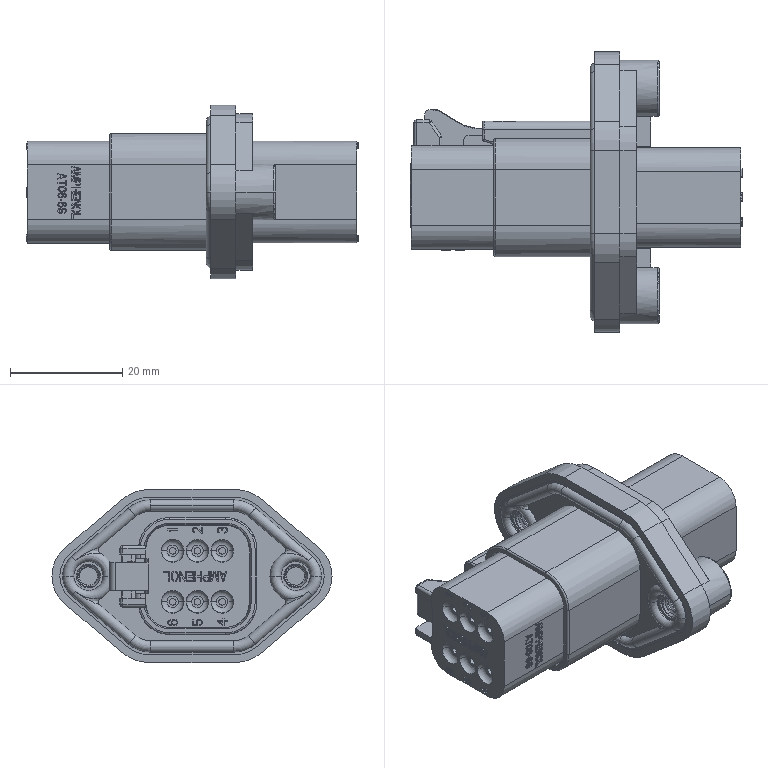Part | NX | features BREP 2 | 2 solids | 1738 faces | box 59.25 x 50 x 31 mm | volume 25746 mm3 | plane 1183 | cylinder 308 | torus 99 | spline 89 | cone 30 | sphere 29 | commonest cylinder face diameters 0.4 x62 3.25 x44 0.2 x24 1.2 x24 2 x17 0.24 x16